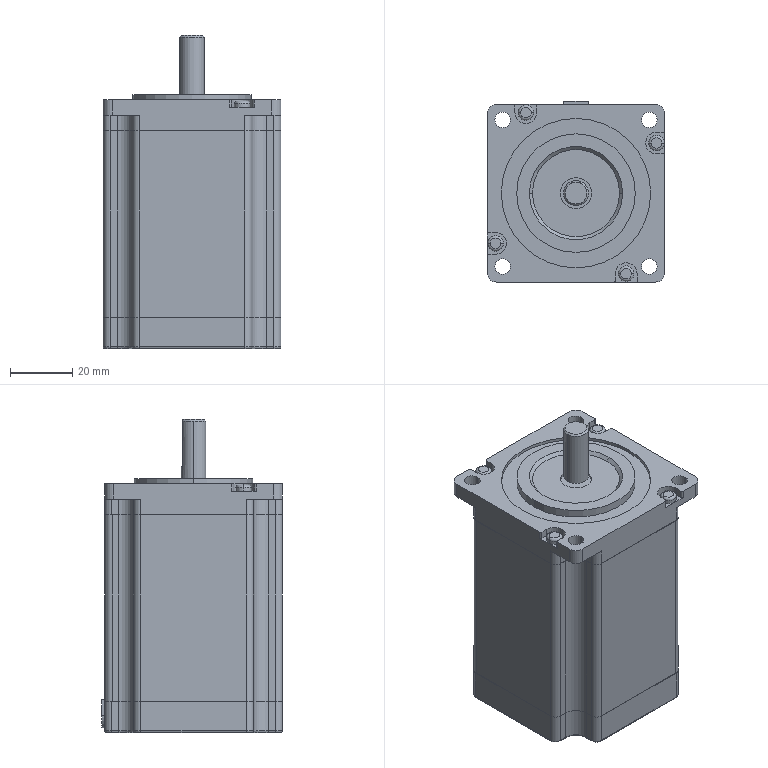Part | SolidWorks | features BaseBody 2 | 2 solids | 216 faces | box 57.15 x 58.15 x 100.6 mm | volume 235224 mm3 | cylinder 100 | plane 79 | torus 32 | cone 5 | commonest cylinder face diameters 4.6 x24 1 x20 5 x16 3 x8 9.5 x8 7 x5